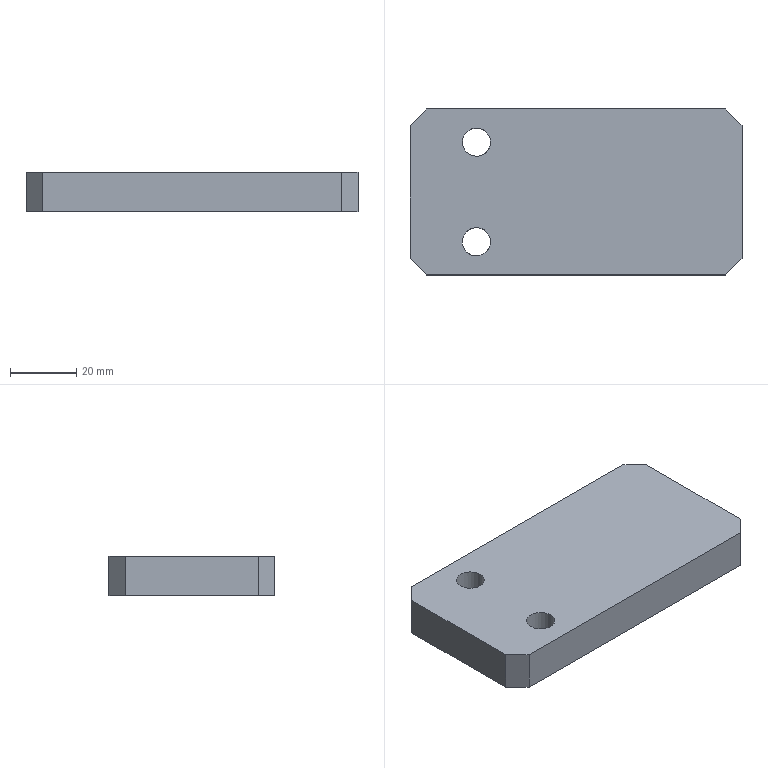Part | NX | features BREP 1 | 1 solid | 12 faces | box 100 x 50 x 12 mm | volume 58038 mm3 | plane 10 | cylinder 2 | commonest cylinder face diameters 8.5 x2
STEP:
#1=CARTESIAN_POINT('',(50.,-20.,12.));
#2=VERTEX_POINT('',#1);
#3=CARTESIAN_POINT('',(50.,20.,12.));
#4=VERTEX_POINT('',#3);
#5=CARTESIAN_POINT('',(50.,25.,12.));
#6=DIRECTION('',(0.,1.,0.));
#7=VECTOR('',#6,1000.);
#8=LINE('',#5,#7);
#9=EDGE_CURVE('',#2,#4,#8,.T.);
#10=ORIENTED_EDGE('',*,*,#9,.F.);
#11=CARTESIAN_POINT('',(50.,-20.,0.));
#12=VERTEX_POINT('',#11);
#13=CARTESIAN_POINT('',(50.,-20.,15.));
#14=DIRECTION('',(0.,0.,-1.));
#15=VECTOR('',#14,1000.);
#16=LINE('',#13,#15);
#17=EDGE_CURVE('',#2,#12,#16,.T.);
#18=ORIENTED_EDGE('',*,*,#17,.T.);
#19=CARTESIAN_POINT('',(50.,20.,0.));
#20=VERTEX_POINT('',#19);
#21=CARTESIAN_POINT('',(50.,25.,0.));
#22=DIRECTION('',(0.,1.,0.));
#23=VECTOR('',#22,1000.);
#24=LINE('',#21,#23);
#25=EDGE_CURVE('',#12,#20,#24,.T.);
#26=ORIENTED_EDGE('',*,*,#25,.T.);
#27=CARTESIAN_POINT('',(50.,20.,15.));
#28=DIRECTION('',(0.,0.,1.));
#29=VECTOR('',#28,1000.);
#30=LINE('',#27,#29);
#31=EDGE_CURVE('',#20,#4,#30,.T.);
#32=ORIENTED_EDGE('',*,*,#31,.T.);
#33=EDGE_LOOP('',(#10,#18,#26,#32));
#34=FACE_BOUND('',#33,.T.);
#35=CARTESIAN_POINT('',(50.,25.,15.));
#36=DIRECTION('',(-1.,0.,0.));
#37=DIRECTION('',(0.,0.,-1.));
#38=AXIS2_PLACEMENT_3D('',#35,#36,#37);
#39=PLANE('',#38);
#40=ADVANCED_FACE('',(#34),#39,.F.);
#41=CARTESIAN_POINT('',(45.,25.,12.));
#42=VERTEX_POINT('',#41);
#43=CARTESIAN_POINT('',(-45.,25.,12.));
#44=VERTEX_POINT('',#43);
#45=CARTESIAN_POINT('',(-50.,25.,12.));
#46=DIRECTION('',(-1.,0.,0.));
#47=VECTOR('',#46,1000.);
#48=LINE('',#45,#47);
#49=EDGE_CURVE('',#42,#44,#48,.T.);
#50=ORIENTED_EDGE('',*,*,#49,.F.);
#51=CARTESIAN_POINT('',(45.,25.,0.));
#52=VERTEX_POINT('',#51);
#53=CARTESIAN_POINT('',(45.,25.,15.));
#54=DIRECTION('',(0.,0.,-1.));
#55=VECTOR('',#54,1000.);
#56=LINE('',#53,#55);
#57=EDGE_CURVE('',#42,#52,#56,.T.);
#58=ORIENTED_EDGE('',*,*,#57,.T.);
#59=CARTESIAN_POINT('',(-45.,25.,0.));
#60=VERTEX_POINT('',#59);
#61=CARTESIAN_POINT('',(-50.,25.,0.));
#62=DIRECTION('',(-1.,0.,0.));
#63=VECTOR('',#62,1000.);
#64=LINE('',#61,#63);
#65=EDGE_CURVE('',#52,#60,#64,.T.);
#66=ORIENTED_EDGE('',*,*,#65,.T.);
#67=CARTESIAN_POINT('',(-45.,25.,15.));
#68=DIRECTION('',(0.,0.,1.));
#69=VECTOR('',#68,1000.);
#70=LINE('',#67,#69);
#71=EDGE_CURVE('',#60,#44,#70,.T.);
#72=ORIENTED_EDGE('',*,*,#71,.T.);
#73=EDGE_LOOP('',(#50,#58,#66,#72));
#74=FACE_BOUND('',#73,.T.);
#75=CARTESIAN_POINT('',(-50.,25.,15.));
#76=DIRECTION('',(0.,-1.,0.));
#77=DIRECTION('',(0.,0.,1.));
#78=AXIS2_PLACEMENT_3D('',#75,#76,#77);
#79=PLANE('',#78);
#80=ADVANCED_FACE('',(#74),#79,.F.);
#81=CARTESIAN_POINT('',(-50.,20.,12.));
#82=VERTEX_POINT('',#81);
#83=CARTESIAN_POINT('',(-50.,-20.,12.));
#84=VERTEX_POINT('',#83);
#85=CARTESIAN_POINT('',(-50.,25.,12.));
#86=DIRECTION('',(0.,-1.,0.));
#87=VECTOR('',#86,1000.);
#88=LINE('',#85,#87);
#89=EDGE_CURVE('',#82,#84,#88,.T.);
#90=ORIENTED_EDGE('',*,*,#89,.F.);
#91=CARTESIAN_POINT('',(-50.,20.,0.));
#92=VERTEX_POINT('',#91);
#93=CARTESIAN_POINT('',(-50.,20.,15.));
#94=DIRECTION('',(0.,0.,-1.));
#95=VECTOR('',#94,1000.);
#96=LINE('',#93,#95);
#97=EDGE_CURVE('',#82,#92,#96,.T.);
#98=ORIENTED_EDGE('',*,*,#97,.T.);
#99=CARTESIAN_POINT('',(-50.,-20.,0.));
#100=VERTEX_POINT('',#99);
#101=CARTESIAN_POINT('',(-50.,25.,0.));
#102=DIRECTION('',(0.,-1.,0.));
#103=VECTOR('',#102,1000.);
#104=LINE('',#101,#103);
#105=EDGE_CURVE('',#92,#100,#104,.T.);
#106=ORIENTED_EDGE('',*,*,#105,.T.);
#107=CARTESIAN_POINT('',(-50.,-20.,15.));
#108=DIRECTION('',(0.,0.,1.));
#109=VECTOR('',#108,1000.);
#110=LINE('',#107,#109);
#111=EDGE_CURVE('',#100,#84,#110,.T.);
#112=ORIENTED_EDGE('',*,*,#111,.T.);
#113=EDGE_LOOP('',(#90,#98,#106,#112));
#114=FACE_BOUND('',#113,.T.);
#115=CARTESIAN_POINT('',(-50.,25.,15.));
#116=DIRECTION('',(1.,0.,0.));
#117=DIRECTION('',(0.,0.,1.));
#118=AXIS2_PLACEMENT_3D('',#115,#116,#117);
#119=PLANE('',#118);
#120=ADVANCED_FACE('',(#114),#119,.F.);
#121=CARTESIAN_POINT('',(-45.,-25.,12.));
#122=VERTEX_POINT('',#121);
#123=CARTESIAN_POINT('',(45.,-25.,12.));
#124=VERTEX_POINT('',#123);
#125=CARTESIAN_POINT('',(-50.,-25.,12.));
#126=DIRECTION('',(1.,0.,0.));
#127=VECTOR('',#126,1000.);
#128=LINE('',#125,#127);
#129=EDGE_CURVE('',#122,#124,#128,.T.);
#130=ORIENTED_EDGE('',*,*,#129,.F.);
#131=CARTESIAN_POINT('',(-45.,-25.,0.));
#132=VERTEX_POINT('',#131);
#133=CARTESIAN_POINT('',(-45.,-25.,15.));
#134=DIRECTION('',(0.,0.,-1.));
#135=VECTOR('',#134,1000.);
#136=LINE('',#133,#135);
#137=EDGE_CURVE('',#122,#132,#136,.T.);
#138=ORIENTED_EDGE('',*,*,#137,.T.);
#139=CARTESIAN_POINT('',(45.,-25.,0.));
#140=VERTEX_POINT('',#139);
#141=CARTESIAN_POINT('',(-50.,-25.,0.));
#142=DIRECTION('',(1.,0.,0.));
#143=VECTOR('',#142,1000.);
#144=LINE('',#141,#143);
#145=EDGE_CURVE('',#132,#140,#144,.T.);
#146=ORIENTED_EDGE('',*,*,#145,.T.);
#147=CARTESIAN_POINT('',(45.,-25.,15.));
#148=DIRECTION('',(0.,0.,1.));
#149=VECTOR('',#148,1000.);
#150=LINE('',#147,#149);
#151=EDGE_CURVE('',#140,#124,#150,.T.);
#152=ORIENTED_EDGE('',*,*,#151,.T.);
#153=EDGE_LOOP('',(#130,#138,#146,#152));
#154=FACE_BOUND('',#153,.T.);
#155=CARTESIAN_POINT('',(-50.,-25.,15.));
#156=DIRECTION('',(0.,1.,0.));
#157=DIRECTION('',(0.,0.,-1.));
#158=AXIS2_PLACEMENT_3D('',#155,#156,#157);
#159=PLANE('',#158);
#160=ADVANCED_FACE('',(#154),#159,.F.);
#161=ORIENTED_EDGE('',*,*,#137,.F.);
#162=CARTESIAN_POINT('',(-45.,-25.,12.));
#163=DIRECTION('',(-0.7071,0.7071,0.));
#164=VECTOR('',#163,1000.);
#165=LINE('',#162,#164);
#166=EDGE_CURVE('',#122,#84,#165,.T.);
#167=ORIENTED_EDGE('',*,*,#166,.T.);
#168=ORIENTED_EDGE('',*,*,#111,.F.);
#169=CARTESIAN_POINT('',(-45.,-25.,0.));
#170=DIRECTION('',(-0.7071,0.7071,0.));
#171=VECTOR('',#170,1000.);
#172=LINE('',#169,#171);
#173=EDGE_CURVE('',#132,#100,#172,.T.);
#174=ORIENTED_EDGE('',*,*,#173,.F.);
#175=EDGE_LOOP('',(#161,#167,#168,#174));
#176=FACE_BOUND('',#175,.T.);
#177=CARTESIAN_POINT('',(-45.,-25.,15.));
#178=DIRECTION('',(0.7071,0.7071,0.));
#179=DIRECTION('',(0.,0.,1.));
#180=AXIS2_PLACEMENT_3D('',#177,#178,#179);
#181=PLANE('',#180);
#182=ADVANCED_FACE('',(#176),#181,.F.);
#183=ORIENTED_EDGE('',*,*,#97,.F.);
#184=CARTESIAN_POINT('',(-50.,20.,12.));
#185=DIRECTION('',(0.7071,0.7071,0.));
#186=VECTOR('',#185,1000.);
#187=LINE('',#184,#186);
#188=EDGE_CURVE('',#82,#44,#187,.T.);
#189=ORIENTED_EDGE('',*,*,#188,.T.);
#190=ORIENTED_EDGE('',*,*,#71,.F.);
#191=CARTESIAN_POINT('',(-50.,20.,0.));
#192=DIRECTION('',(0.7071,0.7071,0.));
#193=VECTOR('',#192,1000.);
#194=LINE('',#191,#193);
#195=EDGE_CURVE('',#92,#60,#194,.T.);
#196=ORIENTED_EDGE('',*,*,#195,.F.);
#197=EDGE_LOOP('',(#183,#189,#190,#196));
#198=FACE_BOUND('',#197,.T.);
#199=CARTESIAN_POINT('',(-50.,20.,15.));
#200=DIRECTION('',(0.7071,-0.7071,0.));
#201=DIRECTION('',(0.,0.,1.));
#202=AXIS2_PLACEMENT_3D('',#199,#200,#201);
#203=PLANE('',#202);
#204=ADVANCED_FACE('',(#198),#203,.F.);
#205=ORIENTED_EDGE('',*,*,#17,.F.);
#206=CARTESIAN_POINT('',(50.,-20.,12.));
#207=DIRECTION('',(-0.7071,-0.7071,0.));
#208=VECTOR('',#207,1000.);
#209=LINE('',#206,#208);
#210=EDGE_CURVE('',#2,#124,#209,.T.);
#211=ORIENTED_EDGE('',*,*,#210,.T.);
#212=ORIENTED_EDGE('',*,*,#151,.F.);
#213=CARTESIAN_POINT('',(50.,-20.,0.));
#214=DIRECTION('',(-0.7071,-0.7071,0.));
#215=VECTOR('',#214,1000.);
#216=LINE('',#213,#215);
#217=EDGE_CURVE('',#12,#140,#216,.T.);
#218=ORIENTED_EDGE('',*,*,#217,.F.);
#219=EDGE_LOOP('',(#205,#211,#212,#218));
#220=FACE_BOUND('',#219,.T.);
#221=CARTESIAN_POINT('',(50.,-20.,15.));
#222=DIRECTION('',(-0.7071,0.7071,0.));
#223=DIRECTION('',(0.,0.,1.));
#224=AXIS2_PLACEMENT_3D('',#221,#222,#223);
#225=PLANE('',#224);
#226=ADVANCED_FACE('',(#220),#225,.F.);
#227=ORIENTED_EDGE('',*,*,#57,.F.);
#228=CARTESIAN_POINT('',(45.,25.,12.));
#229=DIRECTION('',(0.7071,-0.7071,0.));
#230=VECTOR('',#229,1000.);
#231=LINE('',#228,#230);
#232=EDGE_CURVE('',#42,#4,#231,.T.);
#233=ORIENTED_EDGE('',*,*,#232,.T.);
#234=ORIENTED_EDGE('',*,*,#31,.F.);
#235=CARTESIAN_POINT('',(45.,25.,0.));
#236=DIRECTION('',(0.7071,-0.7071,0.));
#237=VECTOR('',#236,1000.);
#238=LINE('',#235,#237);
#239=EDGE_CURVE('',#52,#20,#238,.T.);
#240=ORIENTED_EDGE('',*,*,#239,.F.);
#241=EDGE_LOOP('',(#227,#233,#234,#240));
#242=FACE_BOUND('',#241,.T.);
#243=CARTESIAN_POINT('',(45.,25.,15.));
#244=DIRECTION('',(-0.7071,-0.7071,0.));
#245=DIRECTION('',(0.,0.,1.));
#246=AXIS2_PLACEMENT_3D('',#243,#244,#245);
#247=PLANE('',#246);
#248=ADVANCED_FACE('',(#242),#247,.F.);
#249=CARTESIAN_POINT('',(-25.75,-15.,0.));
#250=VERTEX_POINT('',#249);
#251=CARTESIAN_POINT('',(-30.,-15.,0.));
#252=DIRECTION('',(0.,0.,1.));
#253=DIRECTION('',(1.,0.,0.));
#254=AXIS2_PLACEMENT_3D('',#251,#252,#253);
#255=CIRCLE('',#254,4.25);
#256=EDGE_CURVE('',#250,#250,#255,.T.);
#257=ORIENTED_EDGE('',*,*,#256,.T.);
#258=EDGE_LOOP('',(#257));
#259=FACE_BOUND('',#258,.T.);
#260=CARTESIAN_POINT('',(-25.75,15.,0.));
#261=VERTEX_POINT('',#260);
#262=CARTESIAN_POINT('',(-30.,15.,0.));
#263=DIRECTION('',(0.,0.,1.));
#264=DIRECTION('',(1.,0.,0.));
#265=AXIS2_PLACEMENT_3D('',#262,#263,#264);
#266=CIRCLE('',#265,4.25);
#267=EDGE_CURVE('',#261,#261,#266,.T.);
#268=ORIENTED_EDGE('',*,*,#267,.T.);
#269=EDGE_LOOP('',(#268));
#270=FACE_BOUND('',#269,.T.);
#271=ORIENTED_EDGE('',*,*,#145,.F.);
#272=ORIENTED_EDGE('',*,*,#173,.T.);
#273=ORIENTED_EDGE('',*,*,#105,.F.);
#274=ORIENTED_EDGE('',*,*,#195,.T.);
#275=ORIENTED_EDGE('',*,*,#65,.F.);
#276=ORIENTED_EDGE('',*,*,#239,.T.);
#277=ORIENTED_EDGE('',*,*,#25,.F.);
#278=ORIENTED_EDGE('',*,*,#217,.T.);
#279=EDGE_LOOP('',(#271,#272,#273,#274,#275,#276,#277,#278));
#280=FACE_BOUND('',#279,.T.);
#281=CARTESIAN_POINT('',(0.,0.,0.));
#282=DIRECTION('',(0.,0.,1.));
#283=DIRECTION('',(-1.,0.,0.));
#284=AXIS2_PLACEMENT_3D('',#281,#282,#283);
#285=PLANE('',#284);
#286=ADVANCED_FACE('',(#259,#270,#280),#285,.F.);
#287=CARTESIAN_POINT('',(-30.,-19.25,12.));
#288=VERTEX_POINT('',#287);
#289=CARTESIAN_POINT('',(-30.,-15.,12.));
#290=DIRECTION('',(0.,0.,1.));
#291=DIRECTION('',(0.,-1.,0.));
#292=AXIS2_PLACEMENT_3D('',#289,#290,#291);
#293=CIRCLE('',#292,4.25);
#294=EDGE_CURVE('',#288,#288,#293,.T.);
#295=ORIENTED_EDGE('',*,*,#294,.F.);
#296=EDGE_LOOP('',(#295));
#297=FACE_BOUND('',#296,.T.);
#298=CARTESIAN_POINT('',(-30.,10.75,12.));
#299=VERTEX_POINT('',#298);
#300=CARTESIAN_POINT('',(-30.,15.,12.));
#301=DIRECTION('',(0.,0.,1.));
#302=DIRECTION('',(0.,-1.,0.));
#303=AXIS2_PLACEMENT_3D('',#300,#301,#302);
#304=CIRCLE('',#303,4.25);
#305=EDGE_CURVE('',#299,#299,#304,.T.);
#306=ORIENTED_EDGE('',*,*,#305,.F.);
#307=EDGE_LOOP('',(#306));
#308=FACE_BOUND('',#307,.T.);
#309=ORIENTED_EDGE('',*,*,#129,.T.);
#310=ORIENTED_EDGE('',*,*,#210,.F.);
#311=ORIENTED_EDGE('',*,*,#9,.T.);
#312=ORIENTED_EDGE('',*,*,#232,.F.);
#313=ORIENTED_EDGE('',*,*,#49,.T.);
#314=ORIENTED_EDGE('',*,*,#188,.F.);
#315=ORIENTED_EDGE('',*,*,#89,.T.);
#316=ORIENTED_EDGE('',*,*,#166,.F.);
#317=EDGE_LOOP('',(#309,#310,#311,#312,#313,#314,#315,#316));
#318=FACE_BOUND('',#317,.T.);
#319=CARTESIAN_POINT('',(250.,-380.,12.));
#320=DIRECTION('',(0.,0.,1.));
#321=DIRECTION('',(0.,1.,0.));
#322=AXIS2_PLACEMENT_3D('',#319,#320,#321);
#323=PLANE('',#322);
#324=ADVANCED_FACE('',(#297,#308,#318),#323,.T.);
#325=ORIENTED_EDGE('',*,*,#305,.T.);
#326=EDGE_LOOP('',(#325));
#327=FACE_BOUND('',#326,.T.);
#328=ORIENTED_EDGE('',*,*,#267,.F.);
#329=EDGE_LOOP('',(#328));
#330=FACE_BOUND('',#329,.T.);
#331=CARTESIAN_POINT('',(-30.,15.,12.));
#332=DIRECTION('',(0.,0.,1.));
#333=DIRECTION('',(0.,1.,0.));
#334=AXIS2_PLACEMENT_3D('',#331,#332,#333);
#335=CYLINDRICAL_SURFACE('',#334,4.25);
#336=ADVANCED_FACE('',(#327,#330),#335,.F.);
#337=ORIENTED_EDGE('',*,*,#294,.T.);
#338=EDGE_LOOP('',(#337));
#339=FACE_BOUND('',#338,.T.);
#340=ORIENTED_EDGE('',*,*,#256,.F.);
#341=EDGE_LOOP('',(#340));
#342=FACE_BOUND('',#341,.T.);
#343=CARTESIAN_POINT('',(-30.,-15.,12.));
#344=DIRECTION('',(0.,0.,1.));
#345=DIRECTION('',(0.,1.,0.));
#346=AXIS2_PLACEMENT_3D('',#343,#344,#345);
#347=CYLINDRICAL_SURFACE('',#346,4.25);
#348=ADVANCED_FACE('',(#339,#342),#347,.F.);
#349=CLOSED_SHELL('',(#40,#80,#120,#160,#182,#204,#226,#248,#286,#324,#336,#348));
#350=MANIFOLD_SOLID_BREP('',#349);
#351=(LENGTH_UNIT()NAMED_UNIT(*)SI_UNIT(.MILLI.,.METRE.));
#352=UNCERTAINTY_MEASURE_WITH_UNIT(LENGTH_MEASURE(0.00001),#351,'','');
#353=(NAMED_UNIT(*)PLANE_ANGLE_UNIT()SI_UNIT($,.RADIAN.));
#354=(NAMED_UNIT(*)SI_UNIT($,.STERADIAN.)SOLID_ANGLE_UNIT());
#355=(GEOMETRIC_REPRESENTATION_CONTEXT(3)GLOBAL_UNCERTAINTY_ASSIGNED_CONTEXT((#352))GLOBAL_UNIT_ASSIGNED_CONTEXT((#351,#353,#354))REPRESENTATION_CONTEXT('',''));
#356=ADVANCED_BREP_SHAPE_REPRESENTATION('',(#350),#355);